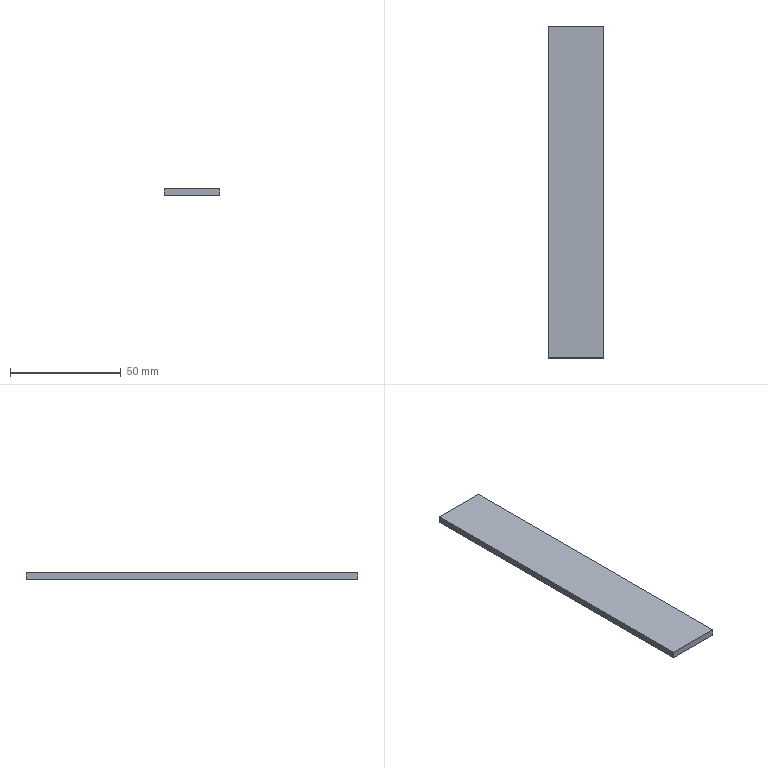Part | SolidWorks | features Extrusion 1 | 1 solid | 6 faces | box 25 x 150 x 3 mm | volume 11250 mm3 | plane 6
STEP:
#1=CARTESIAN_POINT('',(-12.5,75.,1.5));
#2=VERTEX_POINT('',#1);
#3=CARTESIAN_POINT('',(-12.5,-75.,1.5));
#4=VERTEX_POINT('',#3);
#5=CARTESIAN_POINT('',(-12.5,75.,1.5));
#6=DIRECTION('',(0.,-1.,0.));
#7=VECTOR('',#6,1000.);
#8=LINE('',#5,#7);
#9=EDGE_CURVE('',#2,#4,#8,.T.);
#10=ORIENTED_EDGE('',*,*,#9,.F.);
#11=CARTESIAN_POINT('',(-12.5,75.,-1.5));
#12=VERTEX_POINT('',#11);
#13=CARTESIAN_POINT('',(-12.5,75.,-1.5));
#14=DIRECTION('',(0.,0.,1.));
#15=VECTOR('',#14,1000.);
#16=LINE('',#13,#15);
#17=EDGE_CURVE('',#12,#2,#16,.T.);
#18=ORIENTED_EDGE('',*,*,#17,.F.);
#19=CARTESIAN_POINT('',(-12.5,-75.,-1.5));
#20=VERTEX_POINT('',#19);
#21=CARTESIAN_POINT('',(-12.5,75.,-1.5));
#22=DIRECTION('',(0.,-1.,0.));
#23=VECTOR('',#22,1000.);
#24=LINE('',#21,#23);
#25=EDGE_CURVE('',#12,#20,#24,.T.);
#26=ORIENTED_EDGE('',*,*,#25,.T.);
#27=CARTESIAN_POINT('',(-12.5,-75.,-1.5));
#28=DIRECTION('',(0.,0.,1.));
#29=VECTOR('',#28,1000.);
#30=LINE('',#27,#29);
#31=EDGE_CURVE('',#20,#4,#30,.T.);
#32=ORIENTED_EDGE('',*,*,#31,.T.);
#33=EDGE_LOOP('',(#10,#18,#26,#32));
#34=FACE_OUTER_BOUND('',#33,.T.);
#35=CARTESIAN_POINT('',(-12.5,75.,-1.5));
#36=DIRECTION('',(-1.,0.,0.));
#37=DIRECTION('',(0.,0.,1.));
#38=AXIS2_PLACEMENT_3D('',#35,#36,#37);
#39=PLANE('',#38);
#40=ADVANCED_FACE('',(#34),#39,.T.);
#41=CARTESIAN_POINT('',(12.5,75.,1.5));
#42=VERTEX_POINT('',#41);
#43=CARTESIAN_POINT('',(12.5,75.,1.5));
#44=DIRECTION('',(-1.,0.,0.));
#45=VECTOR('',#44,1000.);
#46=LINE('',#43,#45);
#47=EDGE_CURVE('',#42,#2,#46,.T.);
#48=ORIENTED_EDGE('',*,*,#47,.F.);
#49=CARTESIAN_POINT('',(12.5,75.,-1.5));
#50=VERTEX_POINT('',#49);
#51=CARTESIAN_POINT('',(12.5,75.,-1.5));
#52=DIRECTION('',(0.,0.,1.));
#53=VECTOR('',#52,1000.);
#54=LINE('',#51,#53);
#55=EDGE_CURVE('',#50,#42,#54,.T.);
#56=ORIENTED_EDGE('',*,*,#55,.F.);
#57=CARTESIAN_POINT('',(12.5,75.,-1.5));
#58=DIRECTION('',(-1.,0.,0.));
#59=VECTOR('',#58,1000.);
#60=LINE('',#57,#59);
#61=EDGE_CURVE('',#50,#12,#60,.T.);
#62=ORIENTED_EDGE('',*,*,#61,.T.);
#63=ORIENTED_EDGE('',*,*,#17,.T.);
#64=EDGE_LOOP('',(#48,#56,#62,#63));
#65=FACE_OUTER_BOUND('',#64,.T.);
#66=CARTESIAN_POINT('',(12.5,75.,-1.5));
#67=DIRECTION('',(0.,1.,0.));
#68=DIRECTION('',(0.,0.,1.));
#69=AXIS2_PLACEMENT_3D('',#66,#67,#68);
#70=PLANE('',#69);
#71=ADVANCED_FACE('',(#65),#70,.T.);
#72=CARTESIAN_POINT('',(12.5,-75.,1.5));
#73=VERTEX_POINT('',#72);
#74=CARTESIAN_POINT('',(12.5,-75.,1.5));
#75=DIRECTION('',(0.,1.,0.));
#76=VECTOR('',#75,1000.);
#77=LINE('',#74,#76);
#78=EDGE_CURVE('',#73,#42,#77,.T.);
#79=ORIENTED_EDGE('',*,*,#78,.F.);
#80=CARTESIAN_POINT('',(12.5,-75.,-1.5));
#81=VERTEX_POINT('',#80);
#82=CARTESIAN_POINT('',(12.5,-75.,-1.5));
#83=DIRECTION('',(0.,0.,1.));
#84=VECTOR('',#83,1000.);
#85=LINE('',#82,#84);
#86=EDGE_CURVE('',#81,#73,#85,.T.);
#87=ORIENTED_EDGE('',*,*,#86,.F.);
#88=CARTESIAN_POINT('',(12.5,-75.,-1.5));
#89=DIRECTION('',(0.,1.,0.));
#90=VECTOR('',#89,1000.);
#91=LINE('',#88,#90);
#92=EDGE_CURVE('',#81,#50,#91,.T.);
#93=ORIENTED_EDGE('',*,*,#92,.T.);
#94=ORIENTED_EDGE('',*,*,#55,.T.);
#95=EDGE_LOOP('',(#79,#87,#93,#94));
#96=FACE_OUTER_BOUND('',#95,.T.);
#97=CARTESIAN_POINT('',(12.5,-75.,-1.5));
#98=DIRECTION('',(1.,0.,0.));
#99=DIRECTION('',(0.,0.,-1.));
#100=AXIS2_PLACEMENT_3D('',#97,#98,#99);
#101=PLANE('',#100);
#102=ADVANCED_FACE('',(#96),#101,.T.);
#103=CARTESIAN_POINT('',(-12.5,-75.,1.5));
#104=DIRECTION('',(1.,0.,0.));
#105=VECTOR('',#104,1000.);
#106=LINE('',#103,#105);
#107=EDGE_CURVE('',#4,#73,#106,.T.);
#108=ORIENTED_EDGE('',*,*,#107,.F.);
#109=ORIENTED_EDGE('',*,*,#31,.F.);
#110=CARTESIAN_POINT('',(-12.5,-75.,-1.5));
#111=DIRECTION('',(1.,0.,0.));
#112=VECTOR('',#111,1000.);
#113=LINE('',#110,#112);
#114=EDGE_CURVE('',#20,#81,#113,.T.);
#115=ORIENTED_EDGE('',*,*,#114,.T.);
#116=ORIENTED_EDGE('',*,*,#86,.T.);
#117=EDGE_LOOP('',(#108,#109,#115,#116));
#118=FACE_OUTER_BOUND('',#117,.T.);
#119=CARTESIAN_POINT('',(-12.5,-75.,-1.5));
#120=DIRECTION('',(0.,-1.,0.));
#121=DIRECTION('',(0.,0.,-1.));
#122=AXIS2_PLACEMENT_3D('',#119,#120,#121);
#123=PLANE('',#122);
#124=ADVANCED_FACE('',(#118),#123,.T.);
#125=ORIENTED_EDGE('',*,*,#25,.F.);
#126=ORIENTED_EDGE('',*,*,#61,.F.);
#127=ORIENTED_EDGE('',*,*,#92,.F.);
#128=ORIENTED_EDGE('',*,*,#114,.F.);
#129=EDGE_LOOP('',(#125,#126,#127,#128));
#130=FACE_OUTER_BOUND('',#129,.T.);
#131=CARTESIAN_POINT('',(0.,0.,-1.5));
#132=DIRECTION('',(0.,0.,1.));
#133=DIRECTION('',(1.,0.,0.));
#134=AXIS2_PLACEMENT_3D('',#131,#132,#133);
#135=PLANE('',#134);
#136=ADVANCED_FACE('',(#130),#135,.F.);
#137=ORIENTED_EDGE('',*,*,#9,.T.);
#138=ORIENTED_EDGE('',*,*,#107,.T.);
#139=ORIENTED_EDGE('',*,*,#78,.T.);
#140=ORIENTED_EDGE('',*,*,#47,.T.);
#141=EDGE_LOOP('',(#137,#138,#139,#140));
#142=FACE_OUTER_BOUND('',#141,.T.);
#143=CARTESIAN_POINT('',(0.,0.,1.5));
#144=DIRECTION('',(0.,0.,1.));
#145=DIRECTION('',(1.,0.,0.));
#146=AXIS2_PLACEMENT_3D('',#143,#144,#145);
#147=PLANE('',#146);
#148=ADVANCED_FACE('',(#142),#147,.T.);
#149=CLOSED_SHELL('',(#40,#71,#102,#124,#136,#148));
#150=MANIFOLD_SOLID_BREP('',#149);
#151=CARTESIAN_POINT('',(0.,0.,0.));
#152=DIRECTION('',(0.,0.,1.));
#153=DIRECTION('',(1.,0.,0.));
#154=AXIS2_PLACEMENT_3D('',#151,#152,#153);
#155=(LENGTH_UNIT()NAMED_UNIT(*)SI_UNIT(.MILLI.,.METRE.));
#156=UNCERTAINTY_MEASURE_WITH_UNIT(LENGTH_MEASURE(0.00001),#155,'','');
#157=(NAMED_UNIT(*)PLANE_ANGLE_UNIT()SI_UNIT($,.RADIAN.));
#158=(NAMED_UNIT(*)SI_UNIT($,.STERADIAN.)SOLID_ANGLE_UNIT());
#159=(GEOMETRIC_REPRESENTATION_CONTEXT(3)GLOBAL_UNCERTAINTY_ASSIGNED_CONTEXT((#156))GLOBAL_UNIT_ASSIGNED_CONTEXT((#155,#157,#158))REPRESENTATION_CONTEXT('',''));
#160=ADVANCED_BREP_SHAPE_REPRESENTATION('',(#150,#154),#159);